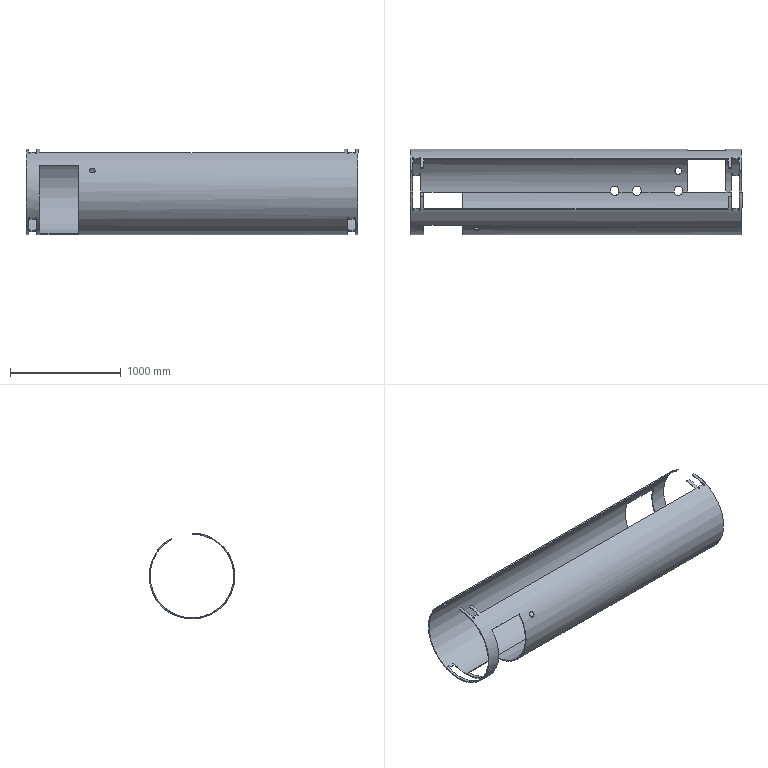Part | SolidWorks | features ICE 10, MirrorPattern 2, 3DProfileFeature 1, CirPattern 1, Extrusion 1, FlatPattern 1, FlattenBends 1, HoleWzd 1, ProcessBends 1, RefPoint 1, SheetMetal 1 | 1 solid | 92 faces | box 3000 x 775 x 774.928 mm | volume 40892506 mm3 | spline 44 | plane 44 | cylinder 4 | commonest cylinder face diameters 759 x2 775 x2